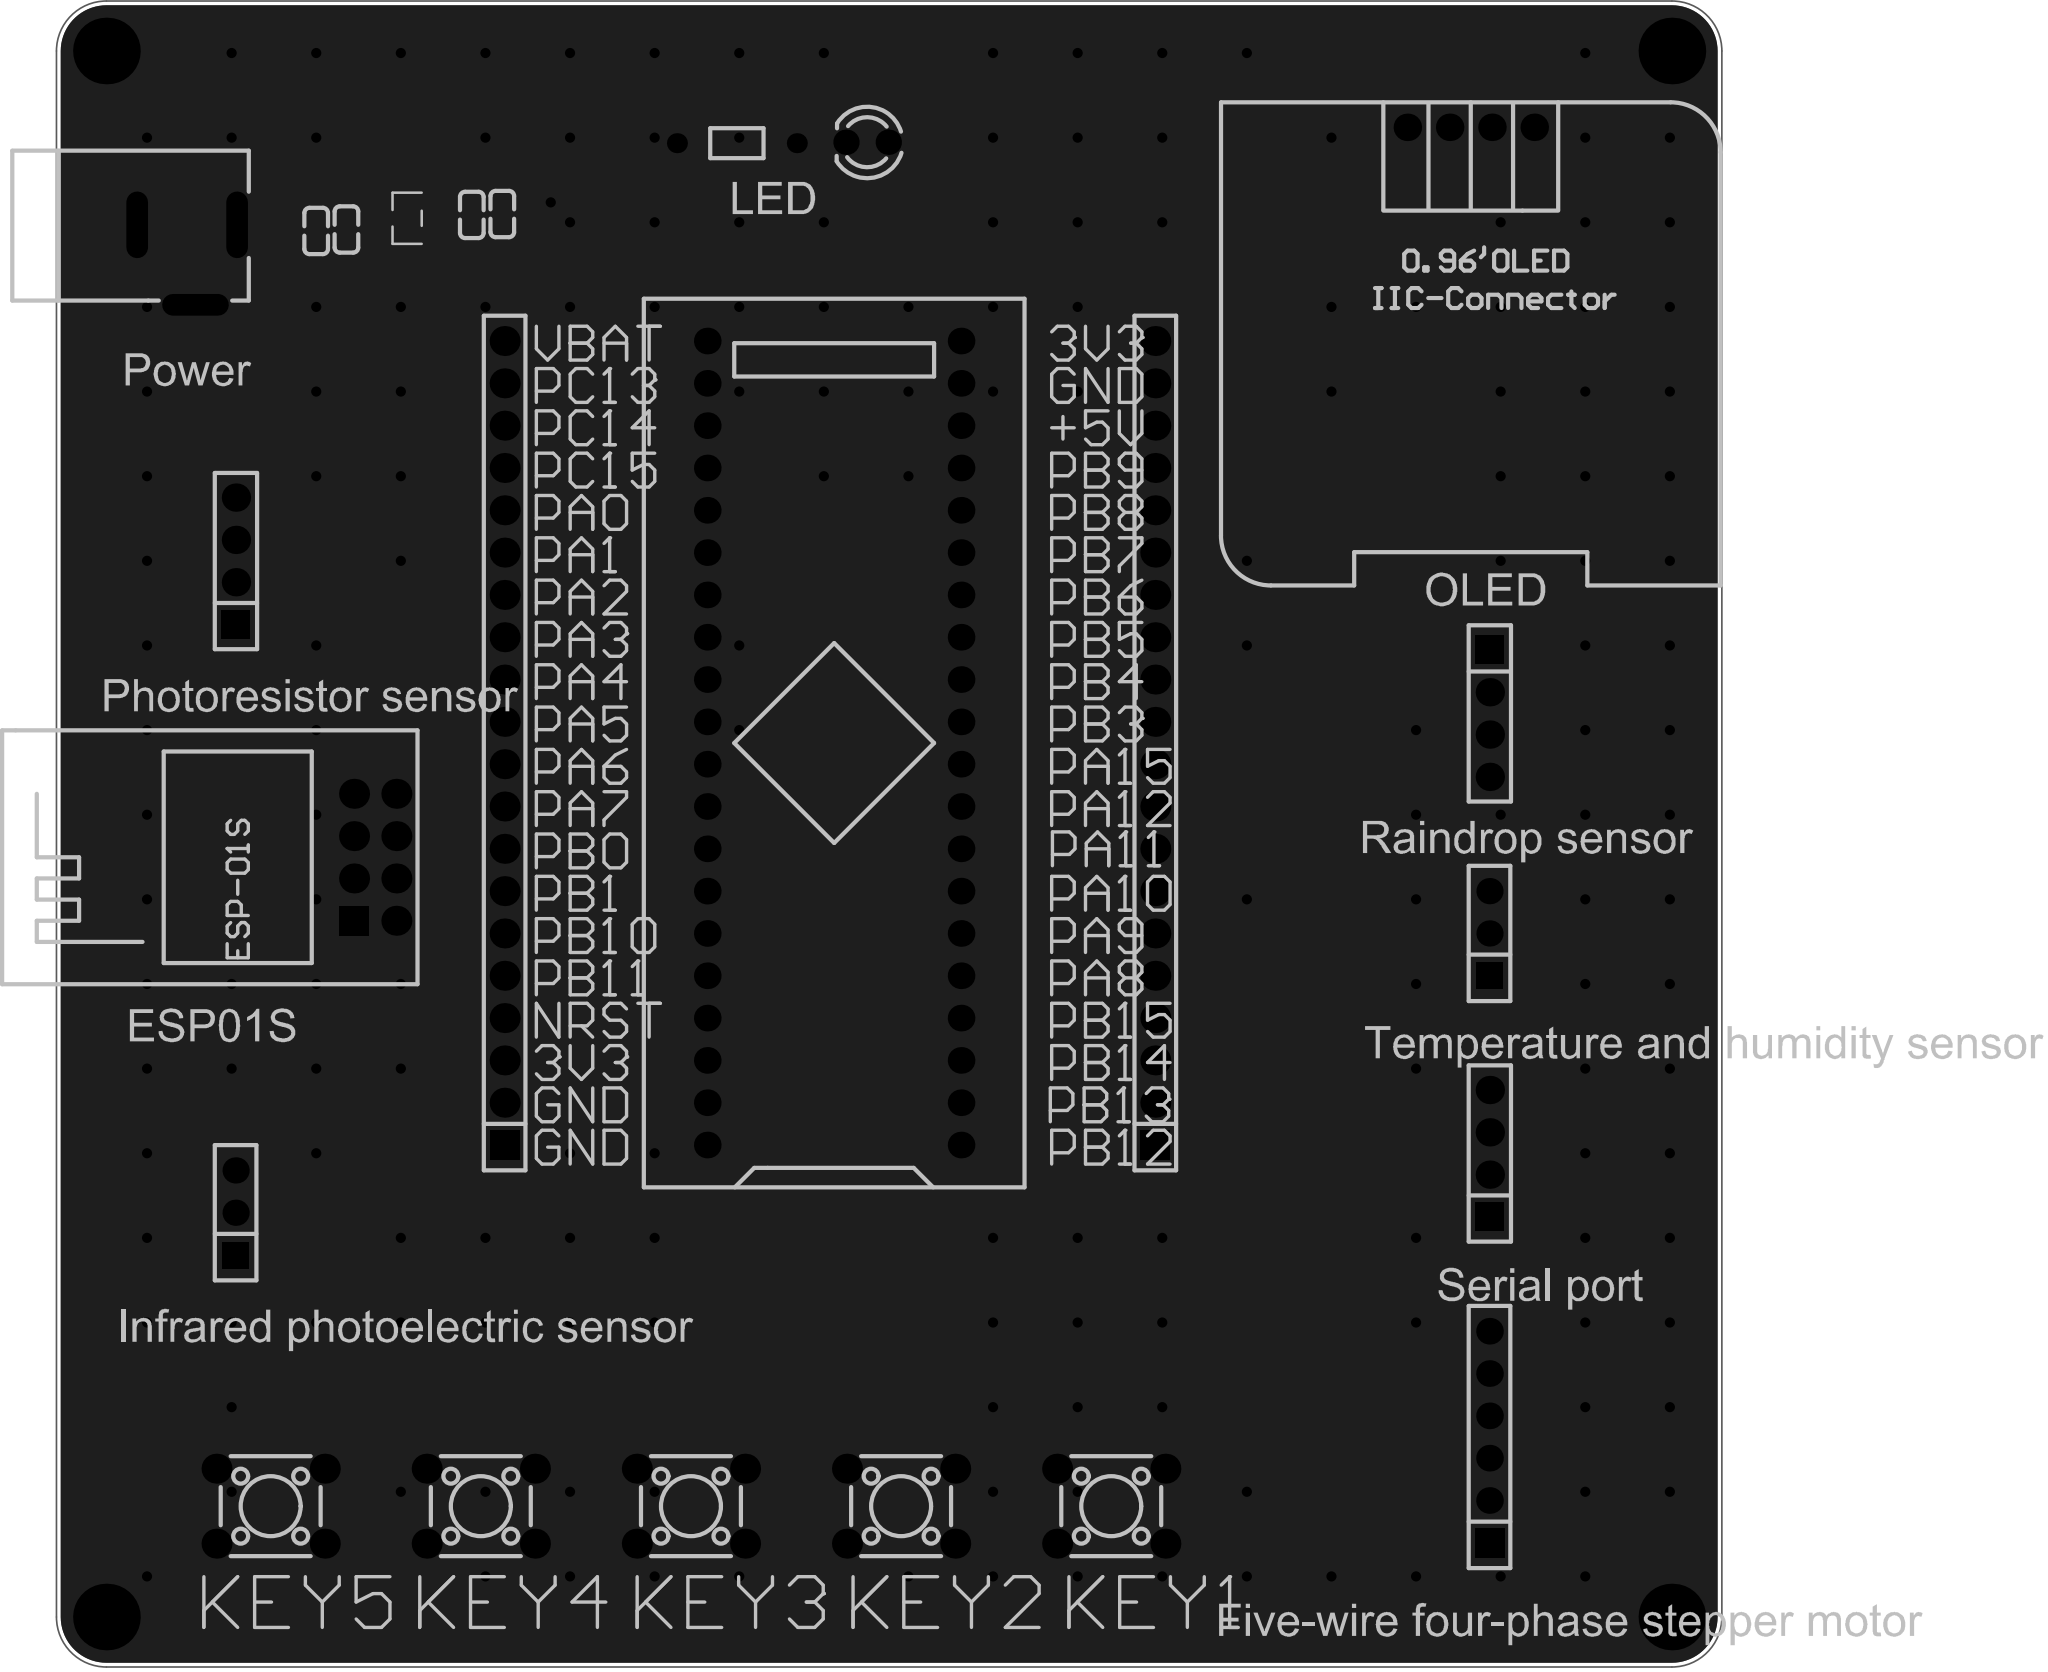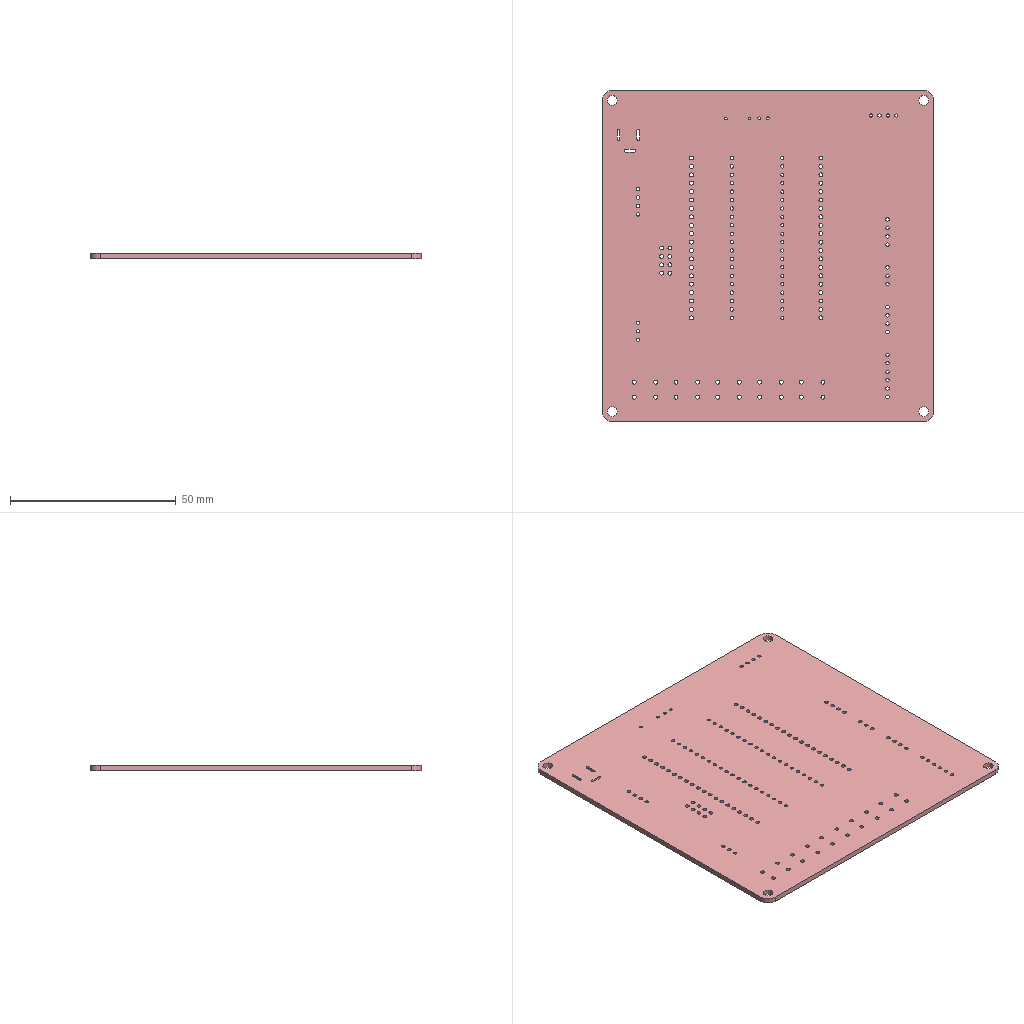Circuit board layout | Altium Designer | box 100 x 100 x 1.6 mm
Layer stack:
# Altium Designer layer stack of  (unit mm; dielectric type: 0 none, 1 core, 2 prepreg, 3 surface material)
index,name,kind,layer,copper_thickness_mm,dielectric_type,dielectric_thickness_mm,dielectric_material,dielectric_constant
0,Top Paste Mask Layer,other,,,,,,
1,Top Silkscreen Layer,other,,,,,,
2,Top Solder Mask Layer,dielectric,,,3,0.01,,3.3
3,Top Layer,copper,Top Layer,0.035,,,,
4,Dielectric1,dielectric,,,3,1.51,FR4,4.5
5,Bottom Layer,copper,Bottom Layer,0.035,,,,
6,Bottom Solder Mask Layer,dielectric,,,3,0.01,,3.3
7,Bottom Silkscreen Layer,other,,,,,,
8,Bottom Paste Mask Layer,other,,,,,,
# drill layer pairs: low layer,high layer
drill_pair,Top Layer,Bottom Layer
Part placement:
Designator,Comment,Layer,Footprint,Center-X(mm),Center-Y(mm),Rotation
U1,STM32F103C8T6-Card,TopLayer,CONN-TH_L53.3-W22.9_STM32F103C8T6-CARD,127.254,134.366,90
H1,,TopLayer,HDR-TH_20P-P2.54-V-F,146.537,134.366,90
H2,,TopLayer,HDR-TH_20P-P2.54-V-F,107.466,134.366,90
C1,10uF,TopLayer,C0603,96.15,165.102,90
C2,100nF,TopLayer,C0603,97.968,165.192,90
C3,10uF,TopLayer,C0603,105.496,166.065,90
C4,100nF,TopLayer,C0603,107.326,166.118,90
DC1,,TopLayer,DC-2.0,88.403,163.071,180
U2,HT7333,TopLayer,SOT-23-3_L2.9-W1.6-P1.90-LS2.8-BR,101.611,165.864,0
H3,,TopLayer,HDR-TH_3P-P2.54-V-F,166.604,122.936,90
H4,,TopLayer,HDR-TH_6P-P2.54-V-F,166.604,92.71,90
H7,,TopLayer,HDR-TH_3P-P2.54-V-F,91.313,106.172,90
H8,,TopLayer,HDR-TH_4P-P2.54-V-F,166.624,136.144,270
H9,,TopLayer,HDR-TH_4P-P2.54-V-F,91.333,145.288,90
H10,,TopLayer,HDR-TH_4P-P2.54-V-F,166.624,109.728,90
LED1,,TopLayer,LED_TH-3mm,129.234,170.429,180
OLED1,,TopLayer,0.96OLED_4P,165.481,171.323,0
R1,220,TopLayer,Res_1/8W,121.412,170.371,180
SW1,,TopLayer,SW-TH_4P-L6.0-W6.0-P4.50-LS6.5,143.891,88.559,0
SW2,,TopLayer,SW-TH_4P-L6.0-W6.0-P4.50-LS6.5,131.273,88.559,0
SW3,,TopLayer,SW-TH_4P-L6.0-W6.0-P4.50-LS6.5,118.654,88.559,0
SW4,,TopLayer,SW-TH_4P-L6.0-W6.0-P4.50-LS6.5,106.036,88.559,0
SW5,,TopLayer,SW-TH_4P-L6.0-W6.0-P4.50-LS6.5,93.418,88.559,0
U3,ESP-01S,TopLayer,WIFIM-TH_ESP-01S,99.695,127.508,90
Pad and via stacks:
# Altium Designer via and pad stacks of  (unit mm). Each distinct definition once, with the count of objects using it.
# via: kind,start_layer,end_layer,hole_mm,diameter_mm,mode(0 simple;1 top-mid-bottom;2 full stack),diameter_per_layer,count,example_net
# pad: kind,layer,hole_mm,hole_type(0 round;1 square;2 slot),plating,top_size,top_shape(1 round;2 rect;3 octagon;9 rounded rect),mid_size,bottom_size,mode,footprint,size_per_layer,count,example
pad,Multi-Layer,3,0,plated,4x4,1,4x4,4x4,0,,,4,1
pad,Multi-Layer,1,0,plated,1.6x1.6,1,1.6x1.6,1.6x1.6,0,CONN-TH_L53.3-W22.9_STM32F103C8T6-CARD,,40,U1.1
pad,Multi-Layer,1.2,0,plated,1.8x1.8,2,1.8x1.8,1.8x1.8,0,HDR-TH_20P-P2.54-V-F,,2,H1.1
pad,Multi-Layer,1.2,0,plated,1.8x1.8,1,1.8x1.8,1.8x1.8,0,HDR-TH_20P-P2.54-V-F,,38,H1.2
pad,Multi-Layer,0.8001,2,plated,4x1.3,1,4x1.3,4x1.3,0,DC-2.0,,3,DC1.2
pad,Multi-Layer,1.02,0,plated,1.575x1.575,1,1.575x1.575,1.575x1.575,0,HDR-TH_3P-P2.54-V-F,,4,H3.3
pad,Multi-Layer,1.02,0,plated,1.575x1.575,2,1.575x1.575,1.575x1.575,0,HDR-TH_3P-P2.54-V-F,,2,H3.1
pad,Multi-Layer,1.02,0,plated,1.6x1.6,1,1.6x1.6,1.6x1.6,0,HDR-TH_6P-P2.54-V-F,,5,H4.6
pad,Multi-Layer,1.02,0,plated,1.8x1.8,2,1.8x1.8,1.8x1.8,0,HDR-TH_6P-P2.54-V-F,,1,H4.1
pad,Multi-Layer,1.1,0,plated,1.7x1.7,2,1.7x1.7,1.7x1.7,0,HDR-TH_4P-P2.54-V-F,,3,H8.1
pad,Multi-Layer,1.1,0,plated,1.7x1.7,1,1.7x1.7,1.7x1.7,0,HDR-TH_4P-P2.54-V-F,,9,H8.2
pad,Multi-Layer,0.9144,0,plated,1.524x1.524,1,1.524x1.524,1.524x1.524,0,LED_TH-3mm,,2,LED1.1
pad,Multi-Layer,1,0,plated,1.65x1.65,1,1.65x1.65,1.65x1.65,0,0.96OLED_4P,,4,OLED1.4
pad,Multi-Layer,0.8001,0,plated,1.199x1.199,1,1.199x1.199,1.199x1.199,0,Res_1/8W,,2,R1.1
pad,Multi-Layer,1.2,0,plated,1.8x1.8,1,1.8x1.8,1.8x1.8,0,SW-TH_4P-L6.0-W6.0-P4.50-LS6.5,,20,SW1.1
pad,Multi-Layer,1.2,0,plated,1.8x1.8,2,1.8x1.8,1.8x1.8,0,WIFIM-TH_ESP-01S,,1,U3.1
pad,Multi-Layer,1.2,0,plated,1.8x1.8,1,1.8x1.8,1.8x1.8,0,WIFIM-TH_ESP-01S,,7,U3.2
pad,Top Layer,0,0,plated,0.8x0.9,2,0.8x0.9,0.8x0.9,0,C0603,,8,C1.2
pad,Top Layer,0,0,plated,1.07x0.6,2,1.07x0.6,1.07x0.6,0,SOT-23-3_L2.9-W1.6-P1.90-LS2.8-BR,,3,U2.1
via,Top Layer,Bottom Layer,0.3048,0.61,0,,177,VCC
Copper pours:
name,layer,net,type(0 solid;1 hatched;2 none)
Bottom Layer-GND,Bottom Layer,GND,0
Top Layer-GND,Top Layer,GND,0